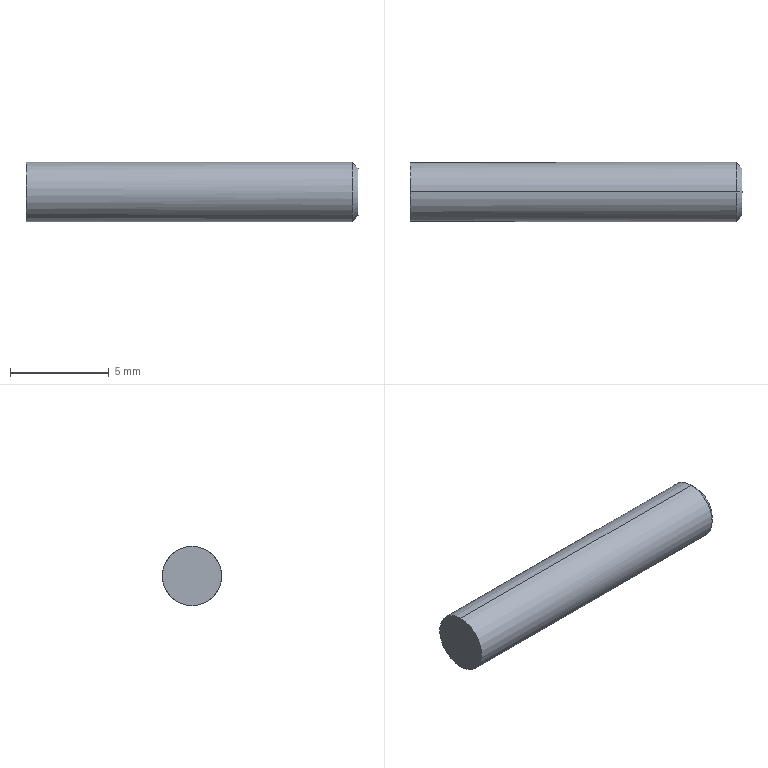Part | STEP file | _X2_751F4E45_X0_MS731-1_X2_8_23 | 1 solid | 6 faces | box 16.8 x 3 x 3 mm | volume 118.356 mm3 | plane 2 | cylinder 2 | cone 2 | commonest cylinder face diameters 3 x2
STEP:
#1=CARTESIAN_POINT('',(0.,0.,0.));
#2=DIRECTION('',(0.,0.,1.));
#3=DIRECTION('',(1.,0.,0.));
#4=AXIS2_PLACEMENT_3D('',#1,#2,#3);
#5=CARTESIAN_POINT('',(7.,13.981,-31.8));
#6=VERTEX_POINT('',#5);
#7=CARTESIAN_POINT('',(7.,13.981,-28.8));
#8=VERTEX_POINT('',#7);
#9=CARTESIAN_POINT('',(7.,13.981,-30.3));
#10=DIRECTION('',(-1.,0.,0.));
#11=DIRECTION('',(0.,0.,-1.));
#12=AXIS2_PLACEMENT_3D('',#9,#10,#11);
#13=CIRCLE('',#12,1.5);
#14=CARTESIAN_POINT('',(7.,13.981,-30.3));
#15=DIRECTION('',(1.,0.,0.));
#16=DIRECTION('',(0.,0.,1.));
#17=AXIS2_PLACEMENT_3D('',#14,#15,#16);
#18=PLANE('',#17);
#19=CARTESIAN_POINT('',(-1.5,0.));
#20=CARTESIAN_POINT('',(-1.5,2.598));
#21=CARTESIAN_POINT('',(0.75,1.299));
#22=CARTESIAN_POINT('',(3.,0.));
#23=CARTESIAN_POINT('',(0.75,-1.299));
#24=CARTESIAN_POINT('',(-1.5,-2.598));
#25=CARTESIAN_POINT('',(-1.5,0.));
#26=(BOUNDED_CURVE()B_SPLINE_CURVE(2,(#19,#20,#21,#22,#23,#24,#25),.UNSPECIFIED.,.T.,.F.)B_SPLINE_CURVE_WITH_KNOTS((1,2,2,2,2,1),(-2.094,0.,2.094,4.189,6.283,8.378),.UNSPECIFIED.)CURVE()GEOMETRIC_REPRESENTATION_ITEM()RATIONAL_B_SPLINE_CURVE((1.,0.5,1.,0.5,1.,0.5,1.))REPRESENTATION_ITEM(''));
#27=(GEOMETRIC_REPRESENTATION_CONTEXT(2)PARAMETRIC_REPRESENTATION_CONTEXT()REPRESENTATION_CONTEXT('',''));
#28=DEFINITIONAL_REPRESENTATION('',(#26),#27);
#29=PCURVE('',#18,#28);
#30=CARTESIAN_POINT('',(7.,13.981,-30.3));
#31=DIRECTION('',(1.,0.,0.));
#32=DIRECTION('',(0.,0.,1.));
#33=AXIS2_PLACEMENT_3D('',#30,#31,#32);
#34=CYLINDRICAL_SURFACE('',#33,1.5);
#35=CARTESIAN_POINT('',(3.142,0.));
#36=DIRECTION('',(-1.,0.));
#37=VECTOR('',#36,1.);
#38=LINE('',#35,#37);
#39=(GEOMETRIC_REPRESENTATION_CONTEXT(2)PARAMETRIC_REPRESENTATION_CONTEXT()REPRESENTATION_CONTEXT('',''));
#40=DEFINITIONAL_REPRESENTATION('',(#38),#39);
#41=PCURVE('',#34,#40);
#42=SURFACE_CURVE('',#13,(#29,#41),.PCURVE_S1.);
#43=EDGE_CURVE('',#6,#8,#42,.T.);
#44=ORIENTED_EDGE('',*,*,#43,.F.);
#45=CARTESIAN_POINT('',(7.,13.981,-30.3));
#46=DIRECTION('',(-1.,0.,0.));
#47=DIRECTION('',(0.,0.,1.));
#48=AXIS2_PLACEMENT_3D('',#45,#46,#47);
#49=CIRCLE('',#48,1.5);
#50=CARTESIAN_POINT('',(1.5,0.));
#51=CARTESIAN_POINT('',(1.5,-2.598));
#52=CARTESIAN_POINT('',(-0.75,-1.299));
#53=CARTESIAN_POINT('',(-3.,0.));
#54=CARTESIAN_POINT('',(-0.75,1.299));
#55=CARTESIAN_POINT('',(1.5,2.598));
#56=CARTESIAN_POINT('',(1.5,0.));
#57=(BOUNDED_CURVE()B_SPLINE_CURVE(2,(#50,#51,#52,#53,#54,#55,#56),.UNSPECIFIED.,.T.,.F.)B_SPLINE_CURVE_WITH_KNOTS((1,2,2,2,2,1),(-2.094,0.,2.094,4.189,6.283,8.378),.UNSPECIFIED.)CURVE()GEOMETRIC_REPRESENTATION_ITEM()RATIONAL_B_SPLINE_CURVE((1.,0.5,1.,0.5,1.,0.5,1.))REPRESENTATION_ITEM(''));
#58=(GEOMETRIC_REPRESENTATION_CONTEXT(2)PARAMETRIC_REPRESENTATION_CONTEXT()REPRESENTATION_CONTEXT('',''));
#59=DEFINITIONAL_REPRESENTATION('',(#57),#58);
#60=PCURVE('',#18,#59);
#61=CARTESIAN_POINT('',(7.,13.981,-30.3));
#62=DIRECTION('',(1.,0.,0.));
#63=DIRECTION('',(0.,0.,1.));
#64=AXIS2_PLACEMENT_3D('',#61,#62,#63);
#65=CYLINDRICAL_SURFACE('',#64,1.5);
#66=CARTESIAN_POINT('',(6.283,0.));
#67=DIRECTION('',(-1.,0.));
#68=VECTOR('',#67,1.);
#69=LINE('',#66,#68);
#70=(GEOMETRIC_REPRESENTATION_CONTEXT(2)PARAMETRIC_REPRESENTATION_CONTEXT()REPRESENTATION_CONTEXT('',''));
#71=DEFINITIONAL_REPRESENTATION('',(#69),#70);
#72=PCURVE('',#65,#71);
#73=SURFACE_CURVE('',#49,(#60,#72),.PCURVE_S1.);
#74=EDGE_CURVE('',#8,#6,#73,.T.);
#75=ORIENTED_EDGE('',*,*,#74,.F.);
#76=EDGE_LOOP('',(#44,#75));
#77=FACE_BOUND('',#76,.F.);
#78=ADVANCED_FACE('',(#77),#18,.F.);
#79=ORIENTED_EDGE('',*,*,#43,.F.);
#80=CARTESIAN_POINT('',(23.5,13.981,-31.8));
#81=VERTEX_POINT('',#80);
#82=CARTESIAN_POINT('',(23.5,13.981,-31.8));
#83=DIRECTION('',(-1.,0.,-0.000000099));
#84=VECTOR('',#83,1.);
#85=LINE('',#82,#84);
#86=CARTESIAN_POINT('',(3.142,16.5));
#87=DIRECTION('',(0.,-1.));
#88=VECTOR('',#87,1.);
#89=LINE('',#86,#88);
#90=(GEOMETRIC_REPRESENTATION_CONTEXT(2)PARAMETRIC_REPRESENTATION_CONTEXT()REPRESENTATION_CONTEXT('',''));
#91=DEFINITIONAL_REPRESENTATION('',(#89),#90);
#92=PCURVE('',#34,#91);
#93=CARTESIAN_POINT('',(3.142,16.5));
#94=DIRECTION('',(0.,-1.));
#95=VECTOR('',#94,1.);
#96=LINE('',#93,#95);
#97=(GEOMETRIC_REPRESENTATION_CONTEXT(2)PARAMETRIC_REPRESENTATION_CONTEXT()REPRESENTATION_CONTEXT('',''));
#98=DEFINITIONAL_REPRESENTATION('',(#96),#97);
#99=PCURVE('',#65,#98);
#100=SURFACE_CURVE('',#85,(#92,#99),.PCURVE_S1.);
#101=EDGE_CURVE('',#81,#6,#100,.T.);
#102=ORIENTED_EDGE('',*,*,#101,.F.);
#103=CARTESIAN_POINT('',(23.5,12.481,-30.3));
#104=VERTEX_POINT('',#103);
#105=CARTESIAN_POINT('',(23.5,13.981,-30.3));
#106=DIRECTION('',(1.,0.,0.));
#107=DIRECTION('',(0.,-1.,0.));
#108=AXIS2_PLACEMENT_3D('',#105,#106,#107);
#109=CIRCLE('',#108,1.5);
#110=CARTESIAN_POINT('',(1.571,16.5));
#111=DIRECTION('',(1.,0.));
#112=VECTOR('',#111,1.);
#113=LINE('',#110,#112);
#114=(GEOMETRIC_REPRESENTATION_CONTEXT(2)PARAMETRIC_REPRESENTATION_CONTEXT()REPRESENTATION_CONTEXT('',''));
#115=DEFINITIONAL_REPRESENTATION('',(#113),#114);
#116=PCURVE('',#34,#115);
#117=CARTESIAN_POINT('',(23.65,13.981,-30.3));
#118=DIRECTION('',(-1.,0.,0.));
#119=DIRECTION('',(0.,-1.,0.));
#120=AXIS2_PLACEMENT_3D('',#117,#118,#119);
#121=CONICAL_SURFACE('',#120,1.35,0.7854);
#122=CARTESIAN_POINT('',(6.283,0.15));
#123=DIRECTION('',(-1.,0.));
#124=VECTOR('',#123,1.);
#125=LINE('',#122,#124);
#126=(GEOMETRIC_REPRESENTATION_CONTEXT(2)PARAMETRIC_REPRESENTATION_CONTEXT()REPRESENTATION_CONTEXT('',''));
#127=DEFINITIONAL_REPRESENTATION('',(#125),#126);
#128=PCURVE('',#121,#127);
#129=SURFACE_CURVE('',#109,(#116,#128),.PCURVE_S1.);
#130=EDGE_CURVE('',#104,#81,#129,.T.);
#131=ORIENTED_EDGE('',*,*,#130,.F.);
#132=CARTESIAN_POINT('',(23.5,13.981,-28.8));
#133=VERTEX_POINT('',#132);
#134=CARTESIAN_POINT('',(23.5,13.981,-30.3));
#135=DIRECTION('',(1.,0.,0.));
#136=DIRECTION('',(0.,0.,1.));
#137=AXIS2_PLACEMENT_3D('',#134,#135,#136);
#138=CIRCLE('',#137,1.5);
#139=CARTESIAN_POINT('',(0.,16.5));
#140=DIRECTION('',(1.,0.));
#141=VECTOR('',#140,1.);
#142=LINE('',#139,#141);
#143=(GEOMETRIC_REPRESENTATION_CONTEXT(2)PARAMETRIC_REPRESENTATION_CONTEXT()REPRESENTATION_CONTEXT('',''));
#144=DEFINITIONAL_REPRESENTATION('',(#142),#143);
#145=PCURVE('',#34,#144);
#146=CARTESIAN_POINT('',(7.854,0.15));
#147=DIRECTION('',(-1.,0.));
#148=VECTOR('',#147,1.);
#149=LINE('',#146,#148);
#150=(GEOMETRIC_REPRESENTATION_CONTEXT(2)PARAMETRIC_REPRESENTATION_CONTEXT()REPRESENTATION_CONTEXT('',''));
#151=DEFINITIONAL_REPRESENTATION('',(#149),#150);
#152=PCURVE('',#121,#151);
#153=SURFACE_CURVE('',#138,(#145,#152),.PCURVE_S1.);
#154=EDGE_CURVE('',#133,#104,#153,.T.);
#155=ORIENTED_EDGE('',*,*,#154,.F.);
#156=CARTESIAN_POINT('',(23.5,13.981,-28.8));
#157=DIRECTION('',(-1.,0.,0.000000099));
#158=VECTOR('',#157,1.);
#159=LINE('',#156,#158);
#160=CARTESIAN_POINT('',(0.,16.5));
#161=DIRECTION('',(0.,-1.));
#162=VECTOR('',#161,1.);
#163=LINE('',#160,#162);
#164=(GEOMETRIC_REPRESENTATION_CONTEXT(2)PARAMETRIC_REPRESENTATION_CONTEXT()REPRESENTATION_CONTEXT('',''));
#165=DEFINITIONAL_REPRESENTATION('',(#163),#164);
#166=PCURVE('',#34,#165);
#167=CARTESIAN_POINT('',(6.283,16.5));
#168=DIRECTION('',(0.,-1.));
#169=VECTOR('',#168,1.);
#170=LINE('',#167,#169);
#171=(GEOMETRIC_REPRESENTATION_CONTEXT(2)PARAMETRIC_REPRESENTATION_CONTEXT()REPRESENTATION_CONTEXT('',''));
#172=DEFINITIONAL_REPRESENTATION('',(#170),#171);
#173=PCURVE('',#65,#172);
#174=SURFACE_CURVE('',#159,(#166,#173),.PCURVE_S1.);
#175=EDGE_CURVE('',#133,#8,#174,.T.);
#176=ORIENTED_EDGE('',*,*,#175,.T.);
#177=EDGE_LOOP('',(#79,#102,#131,#155,#176));
#178=FACE_BOUND('',#177,.T.);
#179=ADVANCED_FACE('',(#178),#34,.T.);
#180=ORIENTED_EDGE('',*,*,#74,.F.);
#181=ORIENTED_EDGE('',*,*,#175,.F.);
#182=CARTESIAN_POINT('',(23.5,15.481,-30.3));
#183=VERTEX_POINT('',#182);
#184=CARTESIAN_POINT('',(23.5,13.981,-30.3));
#185=DIRECTION('',(1.,0.,0.));
#186=DIRECTION('',(0.,1.,0.));
#187=AXIS2_PLACEMENT_3D('',#184,#185,#186);
#188=CIRCLE('',#187,1.5);
#189=CARTESIAN_POINT('',(4.712,16.5));
#190=DIRECTION('',(1.,0.));
#191=VECTOR('',#190,1.);
#192=LINE('',#189,#191);
#193=(GEOMETRIC_REPRESENTATION_CONTEXT(2)PARAMETRIC_REPRESENTATION_CONTEXT()REPRESENTATION_CONTEXT('',''));
#194=DEFINITIONAL_REPRESENTATION('',(#192),#193);
#195=PCURVE('',#65,#194);
#196=CARTESIAN_POINT('',(23.65,13.981,-30.3));
#197=DIRECTION('',(-1.,0.,0.));
#198=DIRECTION('',(0.,-1.,0.));
#199=AXIS2_PLACEMENT_3D('',#196,#197,#198);
#200=CONICAL_SURFACE('',#199,1.35,0.7854);
#201=CARTESIAN_POINT('',(3.142,0.15));
#202=DIRECTION('',(-1.,0.));
#203=VECTOR('',#202,1.);
#204=LINE('',#201,#203);
#205=(GEOMETRIC_REPRESENTATION_CONTEXT(2)PARAMETRIC_REPRESENTATION_CONTEXT()REPRESENTATION_CONTEXT('',''));
#206=DEFINITIONAL_REPRESENTATION('',(#204),#205);
#207=PCURVE('',#200,#206);
#208=SURFACE_CURVE('',#188,(#195,#207),.PCURVE_S1.);
#209=EDGE_CURVE('',#183,#133,#208,.T.);
#210=ORIENTED_EDGE('',*,*,#209,.F.);
#211=CARTESIAN_POINT('',(23.5,13.981,-30.3));
#212=DIRECTION('',(1.,0.,0.));
#213=DIRECTION('',(0.,0.,-1.));
#214=AXIS2_PLACEMENT_3D('',#211,#212,#213);
#215=CIRCLE('',#214,1.5);
#216=CARTESIAN_POINT('',(3.142,16.5));
#217=DIRECTION('',(1.,0.));
#218=VECTOR('',#217,1.);
#219=LINE('',#216,#218);
#220=(GEOMETRIC_REPRESENTATION_CONTEXT(2)PARAMETRIC_REPRESENTATION_CONTEXT()REPRESENTATION_CONTEXT('',''));
#221=DEFINITIONAL_REPRESENTATION('',(#219),#220);
#222=PCURVE('',#65,#221);
#223=CARTESIAN_POINT('',(4.712,0.15));
#224=DIRECTION('',(-1.,0.));
#225=VECTOR('',#224,1.);
#226=LINE('',#223,#225);
#227=(GEOMETRIC_REPRESENTATION_CONTEXT(2)PARAMETRIC_REPRESENTATION_CONTEXT()REPRESENTATION_CONTEXT('',''));
#228=DEFINITIONAL_REPRESENTATION('',(#226),#227);
#229=PCURVE('',#200,#228);
#230=SURFACE_CURVE('',#215,(#222,#229),.PCURVE_S1.);
#231=EDGE_CURVE('',#81,#183,#230,.T.);
#232=ORIENTED_EDGE('',*,*,#231,.F.);
#233=ORIENTED_EDGE('',*,*,#101,.T.);
#234=EDGE_LOOP('',(#180,#181,#210,#232,#233));
#235=FACE_BOUND('',#234,.T.);
#236=ADVANCED_FACE('',(#235),#65,.T.);
#237=ORIENTED_EDGE('',*,*,#231,.T.);
#238=ORIENTED_EDGE('',*,*,#209,.T.);
#239=CARTESIAN_POINT('',(23.8,13.981,-29.1));
#240=VERTEX_POINT('',#239);
#241=CARTESIAN_POINT('',(23.5,13.981,-28.8));
#242=DIRECTION('',(0.7071,0.,-0.7071));
#243=VECTOR('',#242,1.);
#244=LINE('',#241,#243);
#245=CARTESIAN_POINT('',(1.571,0.15));
#246=DIRECTION('',(0.,-1.));
#247=VECTOR('',#246,1.);
#248=LINE('',#245,#247);
#249=(GEOMETRIC_REPRESENTATION_CONTEXT(2)PARAMETRIC_REPRESENTATION_CONTEXT()REPRESENTATION_CONTEXT('',''));
#250=DEFINITIONAL_REPRESENTATION('',(#248),#249);
#251=PCURVE('',#200,#250);
#252=CARTESIAN_POINT('',(7.854,0.15));
#253=DIRECTION('',(0.,-1.));
#254=VECTOR('',#253,1.);
#255=LINE('',#252,#254);
#256=(GEOMETRIC_REPRESENTATION_CONTEXT(2)PARAMETRIC_REPRESENTATION_CONTEXT()REPRESENTATION_CONTEXT('',''));
#257=DEFINITIONAL_REPRESENTATION('',(#255),#256);
#258=PCURVE('',#121,#257);
#259=SURFACE_CURVE('',#244,(#251,#258),.PCURVE_S1.);
#260=EDGE_CURVE('',#133,#240,#259,.T.);
#261=ORIENTED_EDGE('',*,*,#260,.T.);
#262=CARTESIAN_POINT('',(23.8,15.181,-30.3));
#263=VERTEX_POINT('',#262);
#264=CARTESIAN_POINT('',(23.8,13.981,-30.3));
#265=DIRECTION('',(1.,0.,0.));
#266=DIRECTION('',(0.,1.,0.));
#267=AXIS2_PLACEMENT_3D('',#264,#265,#266);
#268=CIRCLE('',#267,1.2);
#269=CARTESIAN_POINT('',(3.142,-0.15));
#270=DIRECTION('',(-1.,0.));
#271=VECTOR('',#270,1.);
#272=LINE('',#269,#271);
#273=(GEOMETRIC_REPRESENTATION_CONTEXT(2)PARAMETRIC_REPRESENTATION_CONTEXT()REPRESENTATION_CONTEXT('',''));
#274=DEFINITIONAL_REPRESENTATION('',(#272),#273);
#275=PCURVE('',#200,#274);
#276=CARTESIAN_POINT('',(23.8,13.981,-30.3));
#277=DIRECTION('',(1.,0.,0.));
#278=DIRECTION('',(0.,0.,1.));
#279=AXIS2_PLACEMENT_3D('',#276,#277,#278);
#280=PLANE('',#279);
#281=CARTESIAN_POINT('',(0.,0.));
#282=DIRECTION('',(0.,-1.));
#283=AXIS2_PLACEMENT_2D('',#281,#282);
#284=CIRCLE('',#283,1.2);
#285=(GEOMETRIC_REPRESENTATION_CONTEXT(2)PARAMETRIC_REPRESENTATION_CONTEXT()REPRESENTATION_CONTEXT('',''));
#286=DEFINITIONAL_REPRESENTATION('',(#284),#285);
#287=PCURVE('',#280,#286);
#288=SURFACE_CURVE('',#268,(#275,#287),.PCURVE_S1.);
#289=EDGE_CURVE('',#263,#240,#288,.T.);
#290=ORIENTED_EDGE('',*,*,#289,.F.);
#291=CARTESIAN_POINT('',(23.8,13.981,-31.5));
#292=VERTEX_POINT('',#291);
#293=CARTESIAN_POINT('',(23.8,13.981,-30.3));
#294=DIRECTION('',(1.,0.,0.));
#295=DIRECTION('',(0.,0.,-1.));
#296=AXIS2_PLACEMENT_3D('',#293,#294,#295);
#297=CIRCLE('',#296,1.2);
#298=CARTESIAN_POINT('',(4.712,-0.15));
#299=DIRECTION('',(-1.,0.));
#300=VECTOR('',#299,1.);
#301=LINE('',#298,#300);
#302=(GEOMETRIC_REPRESENTATION_CONTEXT(2)PARAMETRIC_REPRESENTATION_CONTEXT()REPRESENTATION_CONTEXT('',''));
#303=DEFINITIONAL_REPRESENTATION('',(#301),#302);
#304=PCURVE('',#200,#303);
#305=CARTESIAN_POINT('',(0.,0.));
#306=DIRECTION('',(-1.,0.));
#307=AXIS2_PLACEMENT_2D('',#305,#306);
#308=CIRCLE('',#307,1.2);
#309=(GEOMETRIC_REPRESENTATION_CONTEXT(2)PARAMETRIC_REPRESENTATION_CONTEXT()REPRESENTATION_CONTEXT('',''));
#310=DEFINITIONAL_REPRESENTATION('',(#308),#309);
#311=PCURVE('',#280,#310);
#312=SURFACE_CURVE('',#297,(#304,#311),.PCURVE_S1.);
#313=EDGE_CURVE('',#292,#263,#312,.T.);
#314=ORIENTED_EDGE('',*,*,#313,.F.);
#315=CARTESIAN_POINT('',(23.5,13.981,-31.8));
#316=DIRECTION('',(0.7071,0.,0.7071));
#317=VECTOR('',#316,1.);
#318=LINE('',#315,#317);
#319=CARTESIAN_POINT('',(4.712,0.15));
#320=DIRECTION('',(0.,-1.));
#321=VECTOR('',#320,1.);
#322=LINE('',#319,#321);
#323=(GEOMETRIC_REPRESENTATION_CONTEXT(2)PARAMETRIC_REPRESENTATION_CONTEXT()REPRESENTATION_CONTEXT('',''));
#324=DEFINITIONAL_REPRESENTATION('',(#322),#323);
#325=PCURVE('',#200,#324);
#326=CARTESIAN_POINT('',(4.712,0.15));
#327=DIRECTION('',(0.,-1.));
#328=VECTOR('',#327,1.);
#329=LINE('',#326,#328);
#330=(GEOMETRIC_REPRESENTATION_CONTEXT(2)PARAMETRIC_REPRESENTATION_CONTEXT()REPRESENTATION_CONTEXT('',''));
#331=DEFINITIONAL_REPRESENTATION('',(#329),#330);
#332=PCURVE('',#121,#331);
#333=SURFACE_CURVE('',#318,(#325,#332),.PCURVE_S1.);
#334=EDGE_CURVE('',#81,#292,#333,.T.);
#335=ORIENTED_EDGE('',*,*,#334,.F.);
#336=EDGE_LOOP('',(#237,#238,#261,#290,#314,#335));
#337=FACE_BOUND('',#336,.T.);
#338=ADVANCED_FACE('',(#337),#200,.T.);
#339=ORIENTED_EDGE('',*,*,#154,.T.);
#340=ORIENTED_EDGE('',*,*,#130,.T.);
#341=ORIENTED_EDGE('',*,*,#334,.T.);
#342=CARTESIAN_POINT('',(23.8,12.781,-30.3));
#343=VERTEX_POINT('',#342);
#344=CARTESIAN_POINT('',(23.8,13.981,-30.3));
#345=DIRECTION('',(1.,0.,0.));
#346=DIRECTION('',(0.,-1.,0.));
#347=AXIS2_PLACEMENT_3D('',#344,#345,#346);
#348=CIRCLE('',#347,1.2);
#349=CARTESIAN_POINT('',(6.283,-0.15));
#350=DIRECTION('',(-1.,0.));
#351=VECTOR('',#350,1.);
#352=LINE('',#349,#351);
#353=(GEOMETRIC_REPRESENTATION_CONTEXT(2)PARAMETRIC_REPRESENTATION_CONTEXT()REPRESENTATION_CONTEXT('',''));
#354=DEFINITIONAL_REPRESENTATION('',(#352),#353);
#355=PCURVE('',#121,#354);
#356=CARTESIAN_POINT('',(0.,0.));
#357=DIRECTION('',(0.,1.));
#358=AXIS2_PLACEMENT_2D('',#356,#357);
#359=CIRCLE('',#358,1.2);
#360=(GEOMETRIC_REPRESENTATION_CONTEXT(2)PARAMETRIC_REPRESENTATION_CONTEXT()REPRESENTATION_CONTEXT('',''));
#361=DEFINITIONAL_REPRESENTATION('',(#359),#360);
#362=PCURVE('',#280,#361);
#363=SURFACE_CURVE('',#348,(#355,#362),.PCURVE_S1.);
#364=EDGE_CURVE('',#343,#292,#363,.T.);
#365=ORIENTED_EDGE('',*,*,#364,.F.);
#366=CARTESIAN_POINT('',(23.8,13.981,-30.3));
#367=DIRECTION('',(1.,0.,0.));
#368=DIRECTION('',(0.,0.,1.));
#369=AXIS2_PLACEMENT_3D('',#366,#367,#368);
#370=CIRCLE('',#369,1.2);
#371=CARTESIAN_POINT('',(7.854,-0.15));
#372=DIRECTION('',(-1.,0.));
#373=VECTOR('',#372,1.);
#374=LINE('',#371,#373);
#375=(GEOMETRIC_REPRESENTATION_CONTEXT(2)PARAMETRIC_REPRESENTATION_CONTEXT()REPRESENTATION_CONTEXT('',''));
#376=DEFINITIONAL_REPRESENTATION('',(#374),#375);
#377=PCURVE('',#121,#376);
#378=CARTESIAN_POINT('',(0.,0.));
#379=DIRECTION('',(1.,0.));
#380=AXIS2_PLACEMENT_2D('',#378,#379);
#381=CIRCLE('',#380,1.2);
#382=(GEOMETRIC_REPRESENTATION_CONTEXT(2)PARAMETRIC_REPRESENTATION_CONTEXT()REPRESENTATION_CONTEXT('',''));
#383=DEFINITIONAL_REPRESENTATION('',(#381),#382);
#384=PCURVE('',#280,#383);
#385=SURFACE_CURVE('',#370,(#377,#384),.PCURVE_S1.);
#386=EDGE_CURVE('',#240,#343,#385,.T.);
#387=ORIENTED_EDGE('',*,*,#386,.F.);
#388=ORIENTED_EDGE('',*,*,#260,.F.);
#389=EDGE_LOOP('',(#339,#340,#341,#365,#387,#388));
#390=FACE_BOUND('',#389,.T.);
#391=ADVANCED_FACE('',(#390),#121,.T.);
#392=ORIENTED_EDGE('',*,*,#289,.T.);
#393=ORIENTED_EDGE('',*,*,#386,.T.);
#394=ORIENTED_EDGE('',*,*,#364,.T.);
#395=ORIENTED_EDGE('',*,*,#313,.T.);
#396=EDGE_LOOP('',(#392,#393,#394,#395));
#397=FACE_BOUND('',#396,.T.);
#398=ADVANCED_FACE('',(#397),#280,.T.);
#399=CLOSED_SHELL('',(#78,#179,#236,#338,#391,#398));
#400=MANIFOLD_SOLID_BREP('',#399);
#401=(LENGTH_UNIT()NAMED_UNIT(*)SI_UNIT(.MILLI.,.METRE.));
#402=UNCERTAINTY_MEASURE_WITH_UNIT(LENGTH_MEASURE(0.000002),#401,'','');
#403=(NAMED_UNIT(*)PLANE_ANGLE_UNIT()SI_UNIT($,.RADIAN.));
#404=(NAMED_UNIT(*)SI_UNIT($,.STERADIAN.)SOLID_ANGLE_UNIT());
#405=(GEOMETRIC_REPRESENTATION_CONTEXT(3)GLOBAL_UNCERTAINTY_ASSIGNED_CONTEXT((#402))GLOBAL_UNIT_ASSIGNED_CONTEXT((#401,#403,#404))REPRESENTATION_CONTEXT('',''));
#406=ADVANCED_BREP_SHAPE_REPRESENTATION('',(#4,#400),#405);